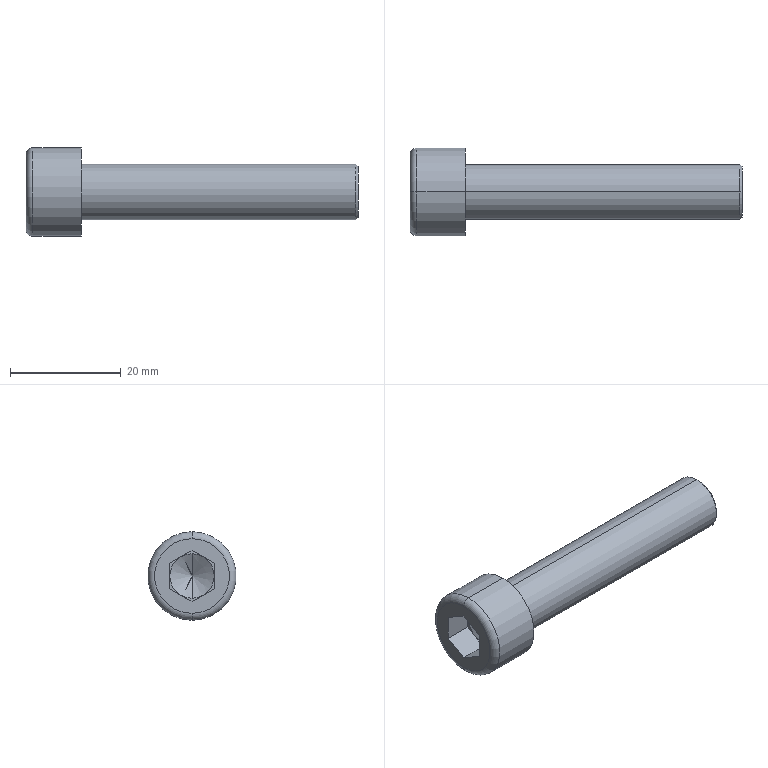Part | SolidWorks | features Fillet 2, RevCut 2, Boss 1, Chamfer 1, Cut 1, Extrusion 1, LPattern 1 | 1 solid | 25 faces | box 60 x 16 x 16 mm | volume 5603 mm3 | plane 15 | cone 4 | cylinder 4 | torus 2 | commonest cylinder face diameters 10 x2 16 x2
STEP:
#1=CARTESIAN_POINT('',(60.,0.,-4.6));
#2=VERTEX_POINT('',#1);
#3=CARTESIAN_POINT('',(60.,0.,4.6));
#4=VERTEX_POINT('',#3);
#5=CARTESIAN_POINT('',(60.,0.,0.));
#6=DIRECTION('',(1.,0.,0.));
#7=DIRECTION('',(0.,0.,-1.));
#8=AXIS2_PLACEMENT_3D('',#5,#6,#7);
#9=CIRCLE('',#8,4.6);
#10=EDGE_CURVE('',#2,#4,#9,.T.);
#11=ORIENTED_EDGE('',*,*,#10,.F.);
#12=CARTESIAN_POINT('',(59.6,0.,-5.));
#13=VERTEX_POINT('',#12);
#14=CARTESIAN_POINT('',(60.,0.,-4.6));
#15=DIRECTION('',(-0.7071,0.,-0.7071));
#16=VECTOR('',#15,1000.);
#17=LINE('',#14,#16);
#18=EDGE_CURVE('',#2,#13,#17,.T.);
#19=ORIENTED_EDGE('',*,*,#18,.T.);
#20=CARTESIAN_POINT('',(59.6,0.,5.));
#21=VERTEX_POINT('',#20);
#22=CARTESIAN_POINT('',(59.6,0.,0.));
#23=DIRECTION('',(-1.,0.,0.));
#24=DIRECTION('',(0.,0.,-1.));
#25=AXIS2_PLACEMENT_3D('',#22,#23,#24);
#26=CIRCLE('',#25,5.);
#27=EDGE_CURVE('',#21,#13,#26,.T.);
#28=ORIENTED_EDGE('',*,*,#27,.F.);
#29=CARTESIAN_POINT('',(60.,0.,4.6));
#30=DIRECTION('',(-0.7071,0.,0.7071));
#31=VECTOR('',#30,1000.);
#32=LINE('',#29,#31);
#33=EDGE_CURVE('',#4,#21,#32,.T.);
#34=ORIENTED_EDGE('',*,*,#33,.F.);
#35=EDGE_LOOP('',(#11,#19,#28,#34));
#36=FACE_OUTER_BOUND('',#35,.T.);
#37=CARTESIAN_POINT('',(60.,0.,0.));
#38=DIRECTION('',(-1.,0.,0.));
#39=DIRECTION('',(0.,0.,1.));
#40=AXIS2_PLACEMENT_3D('',#37,#38,#39);
#41=CONICAL_SURFACE('',#40,4.6,0.7854);
#42=ADVANCED_FACE('',(#36),#41,.T.);
#43=CARTESIAN_POINT('',(0.,0.,6.75));
#44=VERTEX_POINT('',#43);
#45=CARTESIAN_POINT('',(0.,0.,-6.75));
#46=VERTEX_POINT('',#45);
#47=CARTESIAN_POINT('',(0.,0.,0.));
#48=DIRECTION('',(-1.,0.,0.));
#49=DIRECTION('',(0.,0.,-1.));
#50=AXIS2_PLACEMENT_3D('',#47,#48,#49);
#51=CIRCLE('',#50,6.75);
#52=EDGE_CURVE('',#44,#46,#51,.T.);
#53=ORIENTED_EDGE('',*,*,#52,.F.);
#54=CARTESIAN_POINT('',(1.25,0.,8.));
#55=VERTEX_POINT('',#54);
#56=CARTESIAN_POINT('',(1.25,0.,6.75));
#57=DIRECTION('',(0.,1.,0.));
#58=DIRECTION('',(0.,0.,1.));
#59=AXIS2_PLACEMENT_3D('',#56,#57,#58);
#60=CIRCLE('',#59,1.25);
#61=EDGE_CURVE('',#44,#55,#60,.T.);
#62=ORIENTED_EDGE('',*,*,#61,.T.);
#63=CARTESIAN_POINT('',(1.25,0.,-8.));
#64=VERTEX_POINT('',#63);
#65=CARTESIAN_POINT('',(1.25,0.,0.));
#66=DIRECTION('',(1.,0.,0.));
#67=DIRECTION('',(0.,0.,-1.));
#68=AXIS2_PLACEMENT_3D('',#65,#66,#67);
#69=CIRCLE('',#68,8.);
#70=EDGE_CURVE('',#64,#55,#69,.T.);
#71=ORIENTED_EDGE('',*,*,#70,.F.);
#72=CARTESIAN_POINT('',(1.25,0.,-6.75));
#73=DIRECTION('',(0.,-1.,0.));
#74=DIRECTION('',(0.,0.,-1.));
#75=AXIS2_PLACEMENT_3D('',#72,#73,#74);
#76=CIRCLE('',#75,1.25);
#77=EDGE_CURVE('',#46,#64,#76,.T.);
#78=ORIENTED_EDGE('',*,*,#77,.F.);
#79=EDGE_LOOP('',(#53,#62,#71,#78));
#80=FACE_OUTER_BOUND('',#79,.T.);
#81=CARTESIAN_POINT('',(1.25,0.,0.));
#82=DIRECTION('',(1.,0.,0.));
#83=DIRECTION('',(0.,0.,-1.));
#84=AXIS2_PLACEMENT_3D('',#81,#82,#83);
#85=TOROIDAL_SURFACE('',#84,6.75,1.25);
#86=ADVANCED_FACE('',(#80),#85,.T.);
#87=CARTESIAN_POINT('',(7.309,0.,0.));
#88=VERTEX_POINT('',#87);
#89=CARTESIAN_POINT('',(5.,0.,4.));
#90=VERTEX_POINT('',#89);
#91=CARTESIAN_POINT('',(5.,0.,4.));
#92=DIRECTION('',(-0.5,0.,0.866));
#93=VECTOR('',#92,1000.);
#94=LINE('',#91,#93);
#95=EDGE_CURVE('',#88,#90,#94,.T.);
#96=ORIENTED_EDGE('',*,*,#95,.F.);
#97=CARTESIAN_POINT('',(5.,0.,-4.));
#98=VERTEX_POINT('',#97);
#99=CARTESIAN_POINT('',(5.,0.,-4.));
#100=DIRECTION('',(-0.5,0.,-0.866));
#101=VECTOR('',#100,1000.);
#102=LINE('',#99,#101);
#103=EDGE_CURVE('',#88,#98,#102,.T.);
#104=ORIENTED_EDGE('',*,*,#103,.T.);
#105=CARTESIAN_POINT('',(5.,-2.,-3.464));
#106=VERTEX_POINT('',#105);
#107=CARTESIAN_POINT('',(5.,0.,0.));
#108=DIRECTION('',(-1.,0.,0.));
#109=DIRECTION('',(0.,0.,-1.));
#110=AXIS2_PLACEMENT_3D('',#107,#108,#109);
#111=CIRCLE('',#110,4.);
#112=EDGE_CURVE('',#98,#106,#111,.T.);
#113=ORIENTED_EDGE('',*,*,#112,.T.);
#114=CARTESIAN_POINT('',(5.,-4.,0.));
#115=VERTEX_POINT('',#114);
#116=CARTESIAN_POINT('',(5.,0.,0.));
#117=DIRECTION('',(-1.,0.,0.));
#118=DIRECTION('',(0.,0.,-1.));
#119=AXIS2_PLACEMENT_3D('',#116,#117,#118);
#120=CIRCLE('',#119,4.);
#121=EDGE_CURVE('',#106,#115,#120,.T.);
#122=ORIENTED_EDGE('',*,*,#121,.T.);
#123=CARTESIAN_POINT('',(5.,-2.,3.464));
#124=VERTEX_POINT('',#123);
#125=CARTESIAN_POINT('',(5.,0.,0.));
#126=DIRECTION('',(-1.,0.,0.));
#127=DIRECTION('',(0.,0.,-1.));
#128=AXIS2_PLACEMENT_3D('',#125,#126,#127);
#129=CIRCLE('',#128,4.);
#130=EDGE_CURVE('',#115,#124,#129,.T.);
#131=ORIENTED_EDGE('',*,*,#130,.T.);
#132=CARTESIAN_POINT('',(5.,0.,0.));
#133=DIRECTION('',(-1.,0.,0.));
#134=DIRECTION('',(0.,0.,-1.));
#135=AXIS2_PLACEMENT_3D('',#132,#133,#134);
#136=CIRCLE('',#135,4.);
#137=EDGE_CURVE('',#124,#90,#136,.T.);
#138=ORIENTED_EDGE('',*,*,#137,.T.);
#139=EDGE_LOOP('',(#96,#104,#113,#122,#131,#138));
#140=FACE_OUTER_BOUND('',#139,.T.);
#141=CARTESIAN_POINT('',(5.,0.,0.));
#142=DIRECTION('',(-1.,0.,0.));
#143=DIRECTION('',(0.,0.,1.));
#144=AXIS2_PLACEMENT_3D('',#141,#142,#143);
#145=CONICAL_SURFACE('',#144,4.,1.047);
#146=ADVANCED_FACE('',(#140),#145,.F.);
#147=ORIENTED_EDGE('',*,*,#27,.T.);
#148=CARTESIAN_POINT('',(10.,0.,-5.));
#149=VERTEX_POINT('',#148);
#150=CARTESIAN_POINT('',(60.,0.,-5.));
#151=DIRECTION('',(-1.,0.,0.));
#152=VECTOR('',#151,1000.);
#153=LINE('',#150,#152);
#154=EDGE_CURVE('',#13,#149,#153,.T.);
#155=ORIENTED_EDGE('',*,*,#154,.T.);
#156=CARTESIAN_POINT('',(10.,0.,5.));
#157=VERTEX_POINT('',#156);
#158=CARTESIAN_POINT('',(10.,0.,0.));
#159=DIRECTION('',(1.,0.,0.));
#160=DIRECTION('',(0.,0.,-1.));
#161=AXIS2_PLACEMENT_3D('',#158,#159,#160);
#162=CIRCLE('',#161,5.);
#163=EDGE_CURVE('',#149,#157,#162,.T.);
#164=ORIENTED_EDGE('',*,*,#163,.T.);
#165=CARTESIAN_POINT('',(60.,0.,5.));
#166=DIRECTION('',(-1.,0.,0.));
#167=VECTOR('',#166,1000.);
#168=LINE('',#165,#167);
#169=EDGE_CURVE('',#21,#157,#168,.T.);
#170=ORIENTED_EDGE('',*,*,#169,.F.);
#171=EDGE_LOOP('',(#147,#155,#164,#170));
#172=FACE_OUTER_BOUND('',#171,.T.);
#173=CARTESIAN_POINT('',(60.,0.,0.));
#174=DIRECTION('',(-1.,0.,0.));
#175=DIRECTION('',(0.,0.,1.));
#176=AXIS2_PLACEMENT_3D('',#173,#174,#175);
#177=CYLINDRICAL_SURFACE('',#176,5.);
#178=ADVANCED_FACE('',(#172),#177,.T.);
#179=CARTESIAN_POINT('',(10.,0.,-8.));
#180=VERTEX_POINT('',#179);
#181=CARTESIAN_POINT('',(10.,0.,8.));
#182=VERTEX_POINT('',#181);
#183=CARTESIAN_POINT('',(10.,0.,0.));
#184=DIRECTION('',(1.,0.,0.));
#185=DIRECTION('',(0.,0.,-1.));
#186=AXIS2_PLACEMENT_3D('',#183,#184,#185);
#187=CIRCLE('',#186,8.);
#188=EDGE_CURVE('',#180,#182,#187,.T.);
#189=ORIENTED_EDGE('',*,*,#188,.F.);
#190=CARTESIAN_POINT('',(10.,0.,-8.));
#191=DIRECTION('',(-1.,0.,0.));
#192=VECTOR('',#191,1000.);
#193=LINE('',#190,#192);
#194=EDGE_CURVE('',#180,#64,#193,.T.);
#195=ORIENTED_EDGE('',*,*,#194,.T.);
#196=ORIENTED_EDGE('',*,*,#70,.T.);
#197=CARTESIAN_POINT('',(10.,0.,8.));
#198=DIRECTION('',(-1.,0.,0.));
#199=VECTOR('',#198,1000.);
#200=LINE('',#197,#199);
#201=EDGE_CURVE('',#182,#55,#200,.T.);
#202=ORIENTED_EDGE('',*,*,#201,.F.);
#203=EDGE_LOOP('',(#189,#195,#196,#202));
#204=FACE_OUTER_BOUND('',#203,.T.);
#205=CARTESIAN_POINT('',(10.,0.,0.));
#206=DIRECTION('',(-1.,0.,0.));
#207=DIRECTION('',(0.,0.,1.));
#208=AXIS2_PLACEMENT_3D('',#205,#206,#207);
#209=CYLINDRICAL_SURFACE('',#208,8.);
#210=ADVANCED_FACE('',(#204),#209,.T.);
#211=ORIENTED_EDGE('',*,*,#121,.F.);
#212=CARTESIAN_POINT('',(5.,-4.,-2.309));
#213=VERTEX_POINT('',#212);
#214=CARTESIAN_POINT('',(5.,-4.,-2.309));
#215=DIRECTION('',(0.,0.866,-0.5));
#216=VECTOR('',#215,1000.);
#217=LINE('',#214,#216);
#218=EDGE_CURVE('',#213,#106,#217,.T.);
#219=ORIENTED_EDGE('',*,*,#218,.F.);
#220=CARTESIAN_POINT('',(5.,-4.,2.309));
#221=DIRECTION('',(0.,0.,-1.));
#222=VECTOR('',#221,1000.);
#223=LINE('',#220,#222);
#224=EDGE_CURVE('',#115,#213,#223,.T.);
#225=ORIENTED_EDGE('',*,*,#224,.F.);
#226=EDGE_LOOP('',(#211,#219,#225));
#227=FACE_OUTER_BOUND('',#226,.T.);
#228=CARTESIAN_POINT('',(5.,0.,-4.619));
#229=DIRECTION('',(1.,0.,0.));
#230=DIRECTION('',(0.,0.,-1.));
#231=AXIS2_PLACEMENT_3D('',#228,#229,#230);
#232=PLANE('',#231);
#233=ADVANCED_FACE('',(#227),#232,.F.);
#234=ORIENTED_EDGE('',*,*,#130,.F.);
#235=CARTESIAN_POINT('',(5.,-4.,2.309));
#236=VERTEX_POINT('',#235);
#237=CARTESIAN_POINT('',(5.,-4.,2.309));
#238=DIRECTION('',(0.,0.,-1.));
#239=VECTOR('',#238,1000.);
#240=LINE('',#237,#239);
#241=EDGE_CURVE('',#236,#115,#240,.T.);
#242=ORIENTED_EDGE('',*,*,#241,.F.);
#243=CARTESIAN_POINT('',(5.,0.,4.619));
#244=DIRECTION('',(0.,-0.866,-0.5));
#245=VECTOR('',#244,1000.);
#246=LINE('',#243,#245);
#247=EDGE_CURVE('',#124,#236,#246,.T.);
#248=ORIENTED_EDGE('',*,*,#247,.F.);
#249=EDGE_LOOP('',(#234,#242,#248));
#250=FACE_OUTER_BOUND('',#249,.T.);
#251=CARTESIAN_POINT('',(5.,0.,-4.619));
#252=DIRECTION('',(1.,0.,0.));
#253=DIRECTION('',(0.,0.,-1.));
#254=AXIS2_PLACEMENT_3D('',#251,#252,#253);
#255=PLANE('',#254);
#256=ADVANCED_FACE('',(#250),#255,.F.);
#257=ORIENTED_EDGE('',*,*,#137,.F.);
#258=CARTESIAN_POINT('',(5.,0.,4.619));
#259=VERTEX_POINT('',#258);
#260=CARTESIAN_POINT('',(5.,0.,4.619));
#261=DIRECTION('',(0.,-0.866,-0.5));
#262=VECTOR('',#261,1000.);
#263=LINE('',#260,#262);
#264=EDGE_CURVE('',#259,#124,#263,.T.);
#265=ORIENTED_EDGE('',*,*,#264,.F.);
#266=CARTESIAN_POINT('',(5.,2.,3.464));
#267=VERTEX_POINT('',#266);
#268=CARTESIAN_POINT('',(5.,4.,2.309));
#269=DIRECTION('',(0.,-0.866,0.5));
#270=VECTOR('',#269,1000.);
#271=LINE('',#268,#270);
#272=EDGE_CURVE('',#267,#259,#271,.T.);
#273=ORIENTED_EDGE('',*,*,#272,.F.);
#274=CARTESIAN_POINT('',(5.,0.,0.));
#275=DIRECTION('',(-1.,0.,0.));
#276=DIRECTION('',(0.,0.,-1.));
#277=AXIS2_PLACEMENT_3D('',#274,#275,#276);
#278=CIRCLE('',#277,4.);
#279=EDGE_CURVE('',#90,#267,#278,.T.);
#280=ORIENTED_EDGE('',*,*,#279,.F.);
#281=EDGE_LOOP('',(#257,#265,#273,#280));
#282=FACE_OUTER_BOUND('',#281,.T.);
#283=CARTESIAN_POINT('',(5.,0.,-4.619));
#284=DIRECTION('',(1.,0.,0.));
#285=DIRECTION('',(0.,0.,-1.));
#286=AXIS2_PLACEMENT_3D('',#283,#284,#285);
#287=PLANE('',#286);
#288=ADVANCED_FACE('',(#282),#287,.F.);
#289=CARTESIAN_POINT('',(5.,4.,0.));
#290=VERTEX_POINT('',#289);
#291=CARTESIAN_POINT('',(5.,0.,0.));
#292=DIRECTION('',(-1.,0.,0.));
#293=DIRECTION('',(0.,0.,-1.));
#294=AXIS2_PLACEMENT_3D('',#291,#292,#293);
#295=CIRCLE('',#294,4.);
#296=EDGE_CURVE('',#267,#290,#295,.T.);
#297=ORIENTED_EDGE('',*,*,#296,.F.);
#298=CARTESIAN_POINT('',(5.,4.,2.309));
#299=VERTEX_POINT('',#298);
#300=CARTESIAN_POINT('',(5.,4.,2.309));
#301=DIRECTION('',(0.,-0.866,0.5));
#302=VECTOR('',#301,1000.);
#303=LINE('',#300,#302);
#304=EDGE_CURVE('',#299,#267,#303,.T.);
#305=ORIENTED_EDGE('',*,*,#304,.F.);
#306=CARTESIAN_POINT('',(5.,4.,-2.309));
#307=DIRECTION('',(0.,0.,1.));
#308=VECTOR('',#307,1000.);
#309=LINE('',#306,#308);
#310=EDGE_CURVE('',#290,#299,#309,.T.);
#311=ORIENTED_EDGE('',*,*,#310,.F.);
#312=EDGE_LOOP('',(#297,#305,#311));
#313=FACE_OUTER_BOUND('',#312,.T.);
#314=CARTESIAN_POINT('',(5.,0.,-4.619));
#315=DIRECTION('',(1.,0.,0.));
#316=DIRECTION('',(0.,0.,-1.));
#317=AXIS2_PLACEMENT_3D('',#314,#315,#316);
#318=PLANE('',#317);
#319=ADVANCED_FACE('',(#313),#318,.F.);
#320=CARTESIAN_POINT('',(5.,2.,-3.464));
#321=VERTEX_POINT('',#320);
#322=CARTESIAN_POINT('',(5.,0.,0.));
#323=DIRECTION('',(1.,0.,0.));
#324=DIRECTION('',(0.,0.,-1.));
#325=AXIS2_PLACEMENT_3D('',#322,#323,#324);
#326=CIRCLE('',#325,4.);
#327=EDGE_CURVE('',#321,#290,#326,.T.);
#328=ORIENTED_EDGE('',*,*,#327,.T.);
#329=CARTESIAN_POINT('',(5.,4.,-2.309));
#330=VERTEX_POINT('',#329);
#331=CARTESIAN_POINT('',(5.,4.,-2.309));
#332=DIRECTION('',(0.,0.,1.));
#333=VECTOR('',#332,1000.);
#334=LINE('',#331,#333);
#335=EDGE_CURVE('',#330,#290,#334,.T.);
#336=ORIENTED_EDGE('',*,*,#335,.F.);
#337=CARTESIAN_POINT('',(5.,0.,-4.619));
#338=DIRECTION('',(0.,0.866,0.5));
#339=VECTOR('',#338,1000.);
#340=LINE('',#337,#339);
#341=EDGE_CURVE('',#321,#330,#340,.T.);
#342=ORIENTED_EDGE('',*,*,#341,.F.);
#343=EDGE_LOOP('',(#328,#336,#342));
#344=FACE_OUTER_BOUND('',#343,.T.);
#345=CARTESIAN_POINT('',(5.,0.,-4.619));
#346=DIRECTION('',(1.,0.,0.));
#347=DIRECTION('',(0.,0.,-1.));
#348=AXIS2_PLACEMENT_3D('',#345,#346,#347);
#349=PLANE('',#348);
#350=ADVANCED_FACE('',(#344),#349,.F.);
#351=CARTESIAN_POINT('',(5.,0.,0.));
#352=DIRECTION('',(-1.,0.,0.));
#353=DIRECTION('',(0.,0.,-1.));
#354=AXIS2_PLACEMENT_3D('',#351,#352,#353);
#355=CIRCLE('',#354,4.);
#356=EDGE_CURVE('',#321,#98,#355,.T.);
#357=ORIENTED_EDGE('',*,*,#356,.F.);
#358=CARTESIAN_POINT('',(5.,0.,-4.619));
#359=VERTEX_POINT('',#358);
#360=CARTESIAN_POINT('',(5.,0.,-4.619));
#361=DIRECTION('',(0.,0.866,0.5));
#362=VECTOR('',#361,1000.);
#363=LINE('',#360,#362);
#364=EDGE_CURVE('',#359,#321,#363,.T.);
#365=ORIENTED_EDGE('',*,*,#364,.F.);
#366=CARTESIAN_POINT('',(5.,-4.,-2.309));
#367=DIRECTION('',(0.,0.866,-0.5));
#368=VECTOR('',#367,1000.);
#369=LINE('',#366,#368);
#370=EDGE_CURVE('',#106,#359,#369,.T.);
#371=ORIENTED_EDGE('',*,*,#370,.F.);
#372=ORIENTED_EDGE('',*,*,#112,.F.);
#373=EDGE_LOOP('',(#357,#365,#371,#372));
#374=FACE_OUTER_BOUND('',#373,.T.);
#375=CARTESIAN_POINT('',(5.,0.,-4.619));
#376=DIRECTION('',(1.,0.,0.));
#377=DIRECTION('',(0.,0.,-1.));
#378=AXIS2_PLACEMENT_3D('',#375,#376,#377);
#379=PLANE('',#378);
#380=ADVANCED_FACE('',(#374),#379,.F.);
#381=CARTESIAN_POINT('',(0.,0.,0.));
#382=DIRECTION('',(-1.,0.,0.));
#383=DIRECTION('',(0.,0.,-1.));
#384=AXIS2_PLACEMENT_3D('',#381,#382,#383);
#385=CIRCLE('',#384,6.75);
#386=EDGE_CURVE('',#46,#44,#385,.T.);
#387=ORIENTED_EDGE('',*,*,#386,.T.);
#388=ORIENTED_EDGE('',*,*,#52,.T.);
#389=EDGE_LOOP('',(#387,#388));
#390=FACE_OUTER_BOUND('',#389,.T.);
#391=CARTESIAN_POINT('',(0.,-4.,-2.309));
#392=VERTEX_POINT('',#391);
#393=CARTESIAN_POINT('',(0.,0.,-4.619));
#394=VERTEX_POINT('',#393);
#395=CARTESIAN_POINT('',(0.,-4.,-2.309));
#396=DIRECTION('',(0.,0.866,-0.5));
#397=VECTOR('',#396,1000.);
#398=LINE('',#395,#397);
#399=EDGE_CURVE('',#392,#394,#398,.T.);
#400=ORIENTED_EDGE('',*,*,#399,.T.);
#401=CARTESIAN_POINT('',(0.,4.,-2.309));
#402=VERTEX_POINT('',#401);
#403=CARTESIAN_POINT('',(0.,0.,-4.619));
#404=DIRECTION('',(0.,0.866,0.5));
#405=VECTOR('',#404,1000.);
#406=LINE('',#403,#405);
#407=EDGE_CURVE('',#394,#402,#406,.T.);
#408=ORIENTED_EDGE('',*,*,#407,.T.);
#409=CARTESIAN_POINT('',(0.,4.,2.309));
#410=VERTEX_POINT('',#409);
#411=CARTESIAN_POINT('',(0.,4.,-2.309));
#412=DIRECTION('',(0.,0.,1.));
#413=VECTOR('',#412,1000.);
#414=LINE('',#411,#413);
#415=EDGE_CURVE('',#402,#410,#414,.T.);
#416=ORIENTED_EDGE('',*,*,#415,.T.);
#417=CARTESIAN_POINT('',(0.,0.,4.619));
#418=VERTEX_POINT('',#417);
#419=CARTESIAN_POINT('',(0.,4.,2.309));
#420=DIRECTION('',(0.,-0.866,0.5));
#421=VECTOR('',#420,1000.);
#422=LINE('',#419,#421);
#423=EDGE_CURVE('',#410,#418,#422,.T.);
#424=ORIENTED_EDGE('',*,*,#423,.T.);
#425=CARTESIAN_POINT('',(0.,-4.,2.309));
#426=VERTEX_POINT('',#425);
#427=CARTESIAN_POINT('',(0.,0.,4.619));
#428=DIRECTION('',(0.,-0.866,-0.5));
#429=VECTOR('',#428,1000.);
#430=LINE('',#427,#429);
#431=EDGE_CURVE('',#418,#426,#430,.T.);
#432=ORIENTED_EDGE('',*,*,#431,.T.);
#433=CARTESIAN_POINT('',(0.,-4.,2.309));
#434=DIRECTION('',(0.,0.,-1.));
#435=VECTOR('',#434,1000.);
#436=LINE('',#433,#435);
#437=EDGE_CURVE('',#426,#392,#436,.T.);
#438=ORIENTED_EDGE('',*,*,#437,.T.);
#439=EDGE_LOOP('',(#400,#408,#416,#424,#432,#438));
#440=FACE_BOUND('',#439,.T.);
#441=CARTESIAN_POINT('',(0.,0.,0.));
#442=DIRECTION('',(1.,0.,0.));
#443=DIRECTION('',(0.,0.,-1.));
#444=AXIS2_PLACEMENT_3D('',#441,#442,#443);
#445=PLANE('',#444);
#446=ADVANCED_FACE('',(#390,#440),#445,.F.);
#447=CARTESIAN_POINT('',(10.,0.,0.));
#448=DIRECTION('',(1.,0.,0.));
#449=DIRECTION('',(0.,0.,-1.));
#450=AXIS2_PLACEMENT_3D('',#447,#448,#449);
#451=CIRCLE('',#450,8.);
#452=EDGE_CURVE('',#182,#180,#451,.T.);
#453=ORIENTED_EDGE('',*,*,#452,.T.);
#454=ORIENTED_EDGE('',*,*,#188,.T.);
#455=EDGE_LOOP('',(#453,#454));
#456=FACE_OUTER_BOUND('',#455,.T.);
#457=CARTESIAN_POINT('',(10.,0.,0.));
#458=DIRECTION('',(1.,0.,0.));
#459=DIRECTION('',(0.,0.,-1.));
#460=AXIS2_PLACEMENT_3D('',#457,#458,#459);
#461=CIRCLE('',#460,5.);
#462=EDGE_CURVE('',#157,#149,#461,.T.);
#463=ORIENTED_EDGE('',*,*,#462,.F.);
#464=ORIENTED_EDGE('',*,*,#163,.F.);
#465=EDGE_LOOP('',(#463,#464));
#466=FACE_BOUND('',#465,.T.);
#467=CARTESIAN_POINT('',(10.,0.,0.));
#468=DIRECTION('',(1.,0.,0.));
#469=DIRECTION('',(0.,0.,-1.));
#470=AXIS2_PLACEMENT_3D('',#467,#468,#469);
#471=PLANE('',#470);
#472=ADVANCED_FACE('',(#456,#466),#471,.T.);
#473=ORIENTED_EDGE('',*,*,#194,.F.);
#474=ORIENTED_EDGE('',*,*,#452,.F.);
#475=ORIENTED_EDGE('',*,*,#201,.T.);
#476=CARTESIAN_POINT('',(1.25,0.,0.));
#477=DIRECTION('',(1.,0.,0.));
#478=DIRECTION('',(0.,0.,-1.));
#479=AXIS2_PLACEMENT_3D('',#476,#477,#478);
#480=CIRCLE('',#479,8.);
#481=EDGE_CURVE('',#55,#64,#480,.T.);
#482=ORIENTED_EDGE('',*,*,#481,.T.);
#483=EDGE_LOOP('',(#473,#474,#475,#482));
#484=FACE_OUTER_BOUND('',#483,.T.);
#485=CARTESIAN_POINT('',(10.,0.,0.));
#486=DIRECTION('',(-1.,0.,0.));
#487=DIRECTION('',(0.,0.,1.));
#488=AXIS2_PLACEMENT_3D('',#485,#486,#487);
#489=CYLINDRICAL_SURFACE('',#488,8.);
#490=ADVANCED_FACE('',(#484),#489,.T.);
#491=ORIENTED_EDGE('',*,*,#154,.F.);
#492=CARTESIAN_POINT('',(59.6,0.,0.));
#493=DIRECTION('',(-1.,0.,0.));
#494=DIRECTION('',(0.,0.,-1.));
#495=AXIS2_PLACEMENT_3D('',#492,#493,#494);
#496=CIRCLE('',#495,5.);
#497=EDGE_CURVE('',#13,#21,#496,.T.);
#498=ORIENTED_EDGE('',*,*,#497,.T.);
#499=ORIENTED_EDGE('',*,*,#169,.T.);
#500=ORIENTED_EDGE('',*,*,#462,.T.);
#501=EDGE_LOOP('',(#491,#498,#499,#500));
#502=FACE_OUTER_BOUND('',#501,.T.);
#503=CARTESIAN_POINT('',(60.,0.,0.));
#504=DIRECTION('',(-1.,0.,0.));
#505=DIRECTION('',(0.,0.,1.));
#506=AXIS2_PLACEMENT_3D('',#503,#504,#505);
#507=CYLINDRICAL_SURFACE('',#506,5.);
#508=ADVANCED_FACE('',(#502),#507,.T.);
#509=CARTESIAN_POINT('',(60.,0.,0.));
#510=DIRECTION('',(1.,0.,0.));
#511=DIRECTION('',(0.,0.,-1.));
#512=AXIS2_PLACEMENT_3D('',#509,#510,#511);
#513=CIRCLE('',#512,4.6);
#514=EDGE_CURVE('',#4,#2,#513,.T.);
#515=ORIENTED_EDGE('',*,*,#514,.T.);
#516=ORIENTED_EDGE('',*,*,#10,.T.);
#517=EDGE_LOOP('',(#515,#516));
#518=FACE_OUTER_BOUND('',#517,.T.);
#519=CARTESIAN_POINT('',(60.,0.,0.));
#520=DIRECTION('',(1.,0.,0.));
#521=DIRECTION('',(0.,0.,-1.));
#522=AXIS2_PLACEMENT_3D('',#519,#520,#521);
#523=PLANE('',#522);
#524=ADVANCED_FACE('',(#518),#523,.T.);
#525=ORIENTED_EDGE('',*,*,#399,.F.);
#526=CARTESIAN_POINT('',(5.,-4.,-2.309));
#527=DIRECTION('',(-1.,0.,0.));
#528=VECTOR('',#527,1000.);
#529=LINE('',#526,#528);
#530=EDGE_CURVE('',#213,#392,#529,.T.);
#531=ORIENTED_EDGE('',*,*,#530,.F.);
#532=ORIENTED_EDGE('',*,*,#218,.T.);
#533=ORIENTED_EDGE('',*,*,#370,.T.);
#534=CARTESIAN_POINT('',(5.,0.,-4.619));
#535=DIRECTION('',(-1.,0.,0.));
#536=VECTOR('',#535,1000.);
#537=LINE('',#534,#536);
#538=EDGE_CURVE('',#359,#394,#537,.T.);
#539=ORIENTED_EDGE('',*,*,#538,.T.);
#540=EDGE_LOOP('',(#525,#531,#532,#533,#539));
#541=FACE_OUTER_BOUND('',#540,.T.);
#542=CARTESIAN_POINT('',(5.,-4.,-2.309));
#543=DIRECTION('',(0.,0.5,0.866));
#544=DIRECTION('',(0.,-0.866,0.5));
#545=AXIS2_PLACEMENT_3D('',#542,#543,#544);
#546=PLANE('',#545);
#547=ADVANCED_FACE('',(#541),#546,.T.);
#548=ORIENTED_EDGE('',*,*,#407,.F.);
#549=ORIENTED_EDGE('',*,*,#538,.F.);
#550=ORIENTED_EDGE('',*,*,#364,.T.);
#551=ORIENTED_EDGE('',*,*,#341,.T.);
#552=CARTESIAN_POINT('',(5.,4.,-2.309));
#553=DIRECTION('',(-1.,0.,0.));
#554=VECTOR('',#553,1000.);
#555=LINE('',#552,#554);
#556=EDGE_CURVE('',#330,#402,#555,.T.);
#557=ORIENTED_EDGE('',*,*,#556,.T.);
#558=EDGE_LOOP('',(#548,#549,#550,#551,#557));
#559=FACE_OUTER_BOUND('',#558,.T.);
#560=CARTESIAN_POINT('',(5.,0.,-4.619));
#561=DIRECTION('',(0.,-0.5,0.866));
#562=DIRECTION('',(0.,-0.866,-0.5));
#563=AXIS2_PLACEMENT_3D('',#560,#561,#562);
#564=PLANE('',#563);
#565=ADVANCED_FACE('',(#559),#564,.T.);
#566=ORIENTED_EDGE('',*,*,#415,.F.);
#567=ORIENTED_EDGE('',*,*,#556,.F.);
#568=ORIENTED_EDGE('',*,*,#335,.T.);
#569=ORIENTED_EDGE('',*,*,#310,.T.);
#570=CARTESIAN_POINT('',(5.,4.,2.309));
#571=DIRECTION('',(-1.,0.,0.));
#572=VECTOR('',#571,1000.);
#573=LINE('',#570,#572);
#574=EDGE_CURVE('',#299,#410,#573,.T.);
#575=ORIENTED_EDGE('',*,*,#574,.T.);
#576=EDGE_LOOP('',(#566,#567,#568,#569,#575));
#577=FACE_OUTER_BOUND('',#576,.T.);
#578=CARTESIAN_POINT('',(5.,4.,-2.309));
#579=DIRECTION('',(0.,-1.,0.));
#580=DIRECTION('',(0.,0.,-1.));
#581=AXIS2_PLACEMENT_3D('',#578,#579,#580);
#582=PLANE('',#581);
#583=ADVANCED_FACE('',(#577),#582,.T.);
#584=ORIENTED_EDGE('',*,*,#423,.F.);
#585=ORIENTED_EDGE('',*,*,#574,.F.);
#586=ORIENTED_EDGE('',*,*,#304,.T.);
#587=ORIENTED_EDGE('',*,*,#272,.T.);
#588=CARTESIAN_POINT('',(5.,0.,4.619));
#589=DIRECTION('',(-1.,0.,0.));
#590=VECTOR('',#589,1000.);
#591=LINE('',#588,#590);
#592=EDGE_CURVE('',#259,#418,#591,.T.);
#593=ORIENTED_EDGE('',*,*,#592,.T.);
#594=EDGE_LOOP('',(#584,#585,#586,#587,#593));
#595=FACE_OUTER_BOUND('',#594,.T.);
#596=CARTESIAN_POINT('',(5.,4.,2.309));
#597=DIRECTION('',(0.,-0.5,-0.866));
#598=DIRECTION('',(0.,0.866,-0.5));
#599=AXIS2_PLACEMENT_3D('',#596,#597,#598);
#600=PLANE('',#599);
#601=ADVANCED_FACE('',(#595),#600,.T.);
#602=ORIENTED_EDGE('',*,*,#431,.F.);
#603=ORIENTED_EDGE('',*,*,#592,.F.);
#604=ORIENTED_EDGE('',*,*,#264,.T.);
#605=ORIENTED_EDGE('',*,*,#247,.T.);
#606=CARTESIAN_POINT('',(5.,-4.,2.309));
#607=DIRECTION('',(-1.,0.,0.));
#608=VECTOR('',#607,1000.);
#609=LINE('',#606,#608);
#610=EDGE_CURVE('',#236,#426,#609,.T.);
#611=ORIENTED_EDGE('',*,*,#610,.T.);
#612=EDGE_LOOP('',(#602,#603,#604,#605,#611));
#613=FACE_OUTER_BOUND('',#612,.T.);
#614=CARTESIAN_POINT('',(5.,0.,4.619));
#615=DIRECTION('',(0.,0.5,-0.866));
#616=DIRECTION('',(0.,0.866,0.5));
#617=AXIS2_PLACEMENT_3D('',#614,#615,#616);
#618=PLANE('',#617);
#619=ADVANCED_FACE('',(#613),#618,.T.);
#620=ORIENTED_EDGE('',*,*,#437,.F.);
#621=ORIENTED_EDGE('',*,*,#610,.F.);
#622=ORIENTED_EDGE('',*,*,#241,.T.);
#623=ORIENTED_EDGE('',*,*,#224,.T.);
#624=ORIENTED_EDGE('',*,*,#530,.T.);
#625=EDGE_LOOP('',(#620,#621,#622,#623,#624));
#626=FACE_OUTER_BOUND('',#625,.T.);
#627=CARTESIAN_POINT('',(5.,-4.,2.309));
#628=DIRECTION('',(0.,1.,0.));
#629=DIRECTION('',(0.,0.,1.));
#630=AXIS2_PLACEMENT_3D('',#627,#628,#629);
#631=PLANE('',#630);
#632=ADVANCED_FACE('',(#626),#631,.T.);
#633=ORIENTED_EDGE('',*,*,#103,.F.);
#634=ORIENTED_EDGE('',*,*,#95,.T.);
#635=ORIENTED_EDGE('',*,*,#279,.T.);
#636=ORIENTED_EDGE('',*,*,#296,.T.);
#637=ORIENTED_EDGE('',*,*,#327,.F.);
#638=ORIENTED_EDGE('',*,*,#356,.T.);
#639=EDGE_LOOP('',(#633,#634,#635,#636,#637,#638));
#640=FACE_OUTER_BOUND('',#639,.T.);
#641=CARTESIAN_POINT('',(5.,0.,0.));
#642=DIRECTION('',(-1.,0.,0.));
#643=DIRECTION('',(0.,0.,1.));
#644=AXIS2_PLACEMENT_3D('',#641,#642,#643);
#645=CONICAL_SURFACE('',#644,4.,1.047);
#646=ADVANCED_FACE('',(#640),#645,.F.);
#647=ORIENTED_EDGE('',*,*,#61,.F.);
#648=ORIENTED_EDGE('',*,*,#386,.F.);
#649=ORIENTED_EDGE('',*,*,#77,.T.);
#650=ORIENTED_EDGE('',*,*,#481,.F.);
#651=EDGE_LOOP('',(#647,#648,#649,#650));
#652=FACE_OUTER_BOUND('',#651,.T.);
#653=CARTESIAN_POINT('',(1.25,0.,0.));
#654=DIRECTION('',(1.,0.,0.));
#655=DIRECTION('',(0.,0.,-1.));
#656=AXIS2_PLACEMENT_3D('',#653,#654,#655);
#657=TOROIDAL_SURFACE('',#656,6.75,1.25);
#658=ADVANCED_FACE('',(#652),#657,.T.);
#659=ORIENTED_EDGE('',*,*,#18,.F.);
#660=ORIENTED_EDGE('',*,*,#514,.F.);
#661=ORIENTED_EDGE('',*,*,#33,.T.);
#662=ORIENTED_EDGE('',*,*,#497,.F.);
#663=EDGE_LOOP('',(#659,#660,#661,#662));
#664=FACE_OUTER_BOUND('',#663,.T.);
#665=CARTESIAN_POINT('',(60.,0.,0.));
#666=DIRECTION('',(-1.,0.,0.));
#667=DIRECTION('',(0.,0.,1.));
#668=AXIS2_PLACEMENT_3D('',#665,#666,#667);
#669=CONICAL_SURFACE('',#668,4.6,0.7854);
#670=ADVANCED_FACE('',(#664),#669,.T.);
#671=CLOSED_SHELL('',(#42,#86,#146,#178,#210,#233,#256,#288,#319,#350,#380,#446,#472,#490,#508,#524,#547,#565,#583,#601,#619,#632,#646,#658,#670));
#672=MANIFOLD_SOLID_BREP('',#671);
#673=CARTESIAN_POINT('',(0.,0.,0.));
#674=DIRECTION('',(0.,0.,1.));
#675=DIRECTION('',(1.,0.,0.));
#676=AXIS2_PLACEMENT_3D('',#673,#674,#675);
#677=(LENGTH_UNIT()NAMED_UNIT(*)SI_UNIT(.MILLI.,.METRE.));
#678=UNCERTAINTY_MEASURE_WITH_UNIT(LENGTH_MEASURE(0.00001),#677,'','');
#679=(NAMED_UNIT(*)PLANE_ANGLE_UNIT()SI_UNIT($,.RADIAN.));
#680=(NAMED_UNIT(*)SI_UNIT($,.STERADIAN.)SOLID_ANGLE_UNIT());
#681=(GEOMETRIC_REPRESENTATION_CONTEXT(3)GLOBAL_UNCERTAINTY_ASSIGNED_CONTEXT((#678))GLOBAL_UNIT_ASSIGNED_CONTEXT((#677,#679,#680))REPRESENTATION_CONTEXT('',''));
#682=ADVANCED_BREP_SHAPE_REPRESENTATION('',(#672,#676),#681);